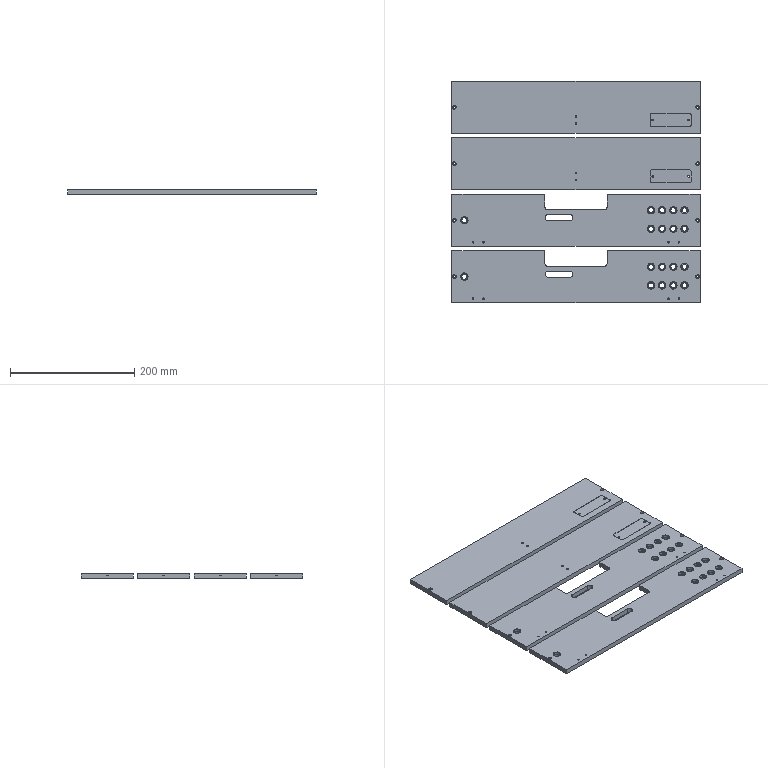CAM job | NX | 3-axis milling | part box 400 x 357 x 8 mm | stock box 404 x 361 x 8 mm
Tools:
number,name,description,diameter,corner_radius,flute_length,length,flutes
2,D4A45,Milling Tool-5 Parameters,4.0,0.0,2.0,2.0,2
6,D6,Milling Tool-5 Parameters,6.0,0.0,50.0,75.0,2
4,D4,Milling Tool-5 Parameters,4.0,0.0,50.0,75.0,2
12,D2,Milling Tool-5 Parameters,2.0,0.0,50.0,75.0,2
15,D1.5,Milling Tool-5 Parameters,1.5,0.0,50.0,75.0,2
Operations:
program,operation,operation_type,tool,method,geometry_group,spindle_rpm,surface_speed,feed_per_tooth,feed_cut,feed_plunge,cut_length_mm,path_length_mm,cut_time_min,machine_time_min
1吸,ZLEVEL_PROFILE_1_COPY_1_COPY_COPY,ZLevelMilling,D4A45,METHOD,A,9500.0,179.0,0.0526,1000.0,100.0,5096.267,16092.928,5.096,6.196
1吸,ZLEVEL_PROFILE_COPY_COPY_1_COPY,ZLevelMilling,D6,METHOD,A,9500.0,179.0,0.1158,2200.0,1000.0,64929.2,66096.128,29.596,29.713
1吸,ZLEVEL_PROFILE_COPY_COPY_1_COPY_COPY,ZLevelMilling,D6,METHOD,A,9500.0,179.0,0.0868,1650.0,1000.0,2775.968,2998.157,1.712,1.735
1吸,HOLE_MILLING_COPY,CylinderMilling,D6,METHOD,A,9500.0,179.0,0.0789,1500.0,100.0,3606.009,5493.034,2.404,2.593
1吸,HOLE_MILLING_COPY_COPY,CylinderMilling,D6,METHOD,A,9500.0,179.0,0.0789,1500.0,100.0,1471.93,3485.555,0.9813,1.183
1吸,HOLE_MILLING,CylinderMilling,D4,METHOD,A,9500.0,179.0,0.0789,1500.0,100.0,579.071,2021.071,0.386,0.5302
1吸,FLOOR_WALL_1,VolumeBased25DMillingOperation,D4,METHOD,A,9500.0,119.0,0.0526,1000.0,100.0,1590.215,1782.522,1.59,1.609
1吸,HOLE_MILLING_COPY_2,CylinderMilling,D2,METHOD,A,9500.0,59.0,0.0526,1000.0,100.0,1276.104,2780.904,1.276,1.427
1吸,HOLE_MILLING_COPY_COPY_1,CylinderMilling,D1.5,METHOD,A,9500.0,44.0,0.0368,700.0,100.0,2157.523,4016.976,3.082,3.268
1吸,HOLE_MILLING_COPY_COPY_1_COPY,CylinderMilling,D1.5,METHOD,A,9500.0,44.0,0.0368,700.0,100.0,668.852,1164.564,0.9555,1.005
1吸,ZLEVEL_PROFILE_COPY_COPY_COPY_COPY_COPY,ZLevelMilling,D4,MILL_FINISH,A,9500.0,119.0,0.0632,1200.0,1000.0,4029.806,5041.794,3.36,3.461